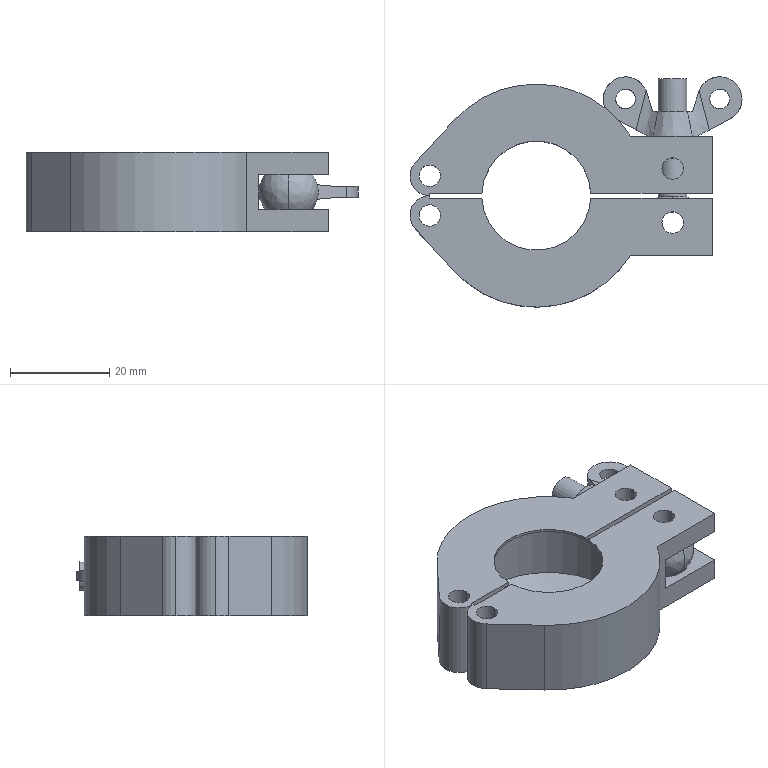Part | SolidWorks | features BaseBody 4 | 4 solids | 142 faces | box 67 x 46.5 x 16 mm | volume 18231 mm3 | cylinder 55 | cone 44 | plane 37 | spline 6 | commonest cylinder face diameters 4.134 x20 4.33 x12 4 x4 8 x4 22 x4 9 x3